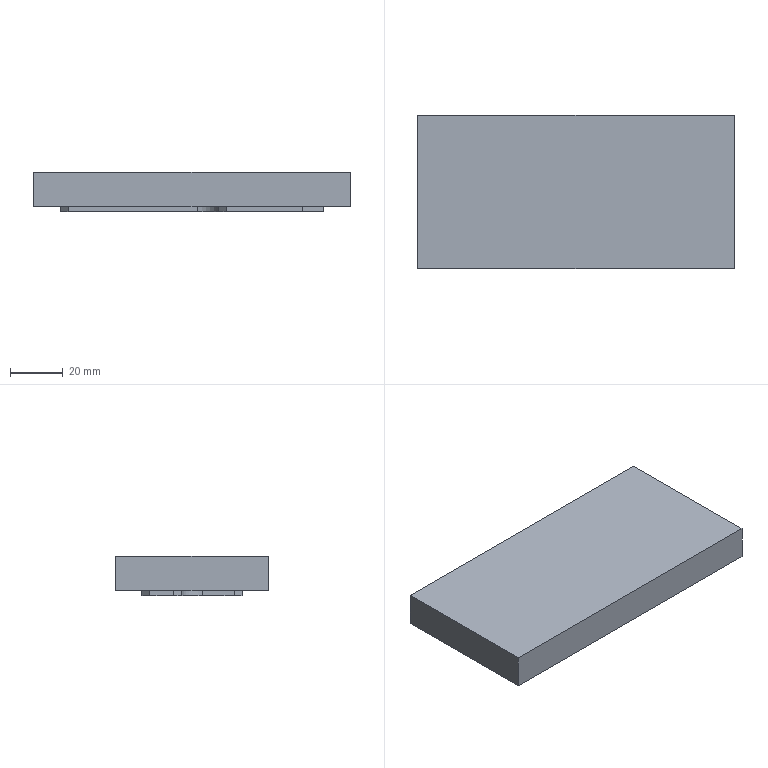NC program | NX | posted with a generic post | part box 120 x 58 x 15 mm
Lines 953 to 1801 of 3687:
(ZLEVEL_PROFILE_COPY_COPY_COPY , TOOL : D3)
N1880 T17 M6
N1882 G54
N1884 G17 G0 G90 X-14.524 Y12.25 S9500 M3
N1886 G43 Z30. H17
N1888 Z1.
N1890 G94 G1 X6.072 Z-0.079 F1000.
N1892 X6.264 Y12.287 Z-0.09
N1894 X6.517 Y12.443 Z-0.105
N1896 X6.691 Y12.683 Z-0.121
N1898 X6.759 Y12.971 Z-0.136
N1900 X6.713 Y13.264 Z-0.152
N1902 X6.591 Y13.477 Z-0.165
N1904 X6.382 Y13.657 Z-0.179
N1906 X6.123 Y13.75 Z-0.194
N1908 X6. Z-0.2
N1910 X-44. F1200.
N1912 G3 X-44.75 Y13. R0.75
N1914 X-44. Y12.25 R0.75
N1916 G1 X6.
N1918 G3 X6.75 Y13. R0.75
N1920 X6. Y13.75 R0.75
N1922 G1 X-5.458 Z-0.4
N1924 X-44.
N1926 G3 X-44.75 Y13. R0.75
N1928 X-44. Y12.25 R0.75
N1930 G1 X6.
N1932 G3 X6.75 Y13. R0.75
N1934 X6. Y13.75 R0.75
N1936 G1 X-5.458 Z-0.6
N1938 X-44.
N1940 G3 X-44.75 Y13. R0.75
N1942 X-44. Y12.25 R0.75
N1944 G1 X6.
N1946 G3 X6.75 Y13. R0.75
N1948 X6. Y13.75 R0.75
N1950 G1 X-5.458 Z-0.8
N1952 X-44.
N1954 G3 X-44.75 Y13. R0.75
N1956 X-44. Y12.25 R0.75
N1958 G1 X6.
N1960 G3 X6.75 Y13. R0.75
N1962 X6. Y13.75 R0.75
N1964 G1 X-5.458 Z-1.
N1966 X-44.
N1968 G3 X-44.75 Y13. R0.75
N1970 X-44. Y12.25 R0.75
N1972 G1 X6.
N1974 G3 X6.75 Y13. R0.75
N1976 X6. Y13.75 R0.75
N1978 G1 X-5.458 Z-1.2
N1980 X-44.
N1982 G3 X-44.75 Y13. R0.75
N1984 X-44. Y12.25 R0.75
N1986 G1 X6.
N1988 G3 X6.75 Y13. R0.75
N1990 X6. Y13.75 R0.75
N1992 G1 X-5.458 Z-1.4
N1994 X-44.
N1996 G3 X-44.75 Y13. R0.75
N1998 X-44. Y12.25 R0.75
N2000 G1 X6.
N2002 G3 X6.75 Y13. R0.75
N2004 X6. Y13.75 R0.75
N2006 G1 X-5.458 Z-1.6
N2008 X-44.
N2010 G3 X-44.75 Y13. R0.75
N2012 X-44. Y12.25 R0.75
N2014 G1 X6.
N2016 G3 X6.75 Y13. R0.75
N2018 X6. Y13.75 R0.75
N2020 G1 X-5.458 Z-1.8
N2022 X-44.
N2024 G3 X-44.75 Y13. R0.75
N2026 X-44. Y12.25 R0.75
N2028 G1 X6.
N2030 G3 X6.75 Y13. R0.75
N2032 X6. Y13.75 R0.75
N2034 G1 X-5.458 Z-2.
N2036 X-44.
N2038 G3 X-44.75 Y13. R0.75
N2040 X-44. Y12.25 R0.75
N2042 G1 X6.
N2044 G3 X6.75 Y13. R0.75
N2046 X6. Y13.75 R0.75
N2048 G1 X-5.458 Z-2.2
N2050 X-44.
N2052 G3 X-44.75 Y13. R0.75
N2054 X-44. Y12.25 R0.75
N2056 G1 X6.
N2058 G3 X6.75 Y13. R0.75
N2060 X6. Y13.75 R0.75
N2062 G1 X-5.458 Z-2.4
N2064 X-44.
N2066 G3 X-44.75 Y13. R0.75
N2068 X-44. Y12.25 R0.75
N2070 G1 X6.
N2072 G3 X6.75 Y13. R0.75
N2074 X6. Y13.75 R0.75
N2076 G1 X-5.458 Z-2.6
N2078 X-44.
N2080 G3 X-44.75 Y13. R0.75
N2082 X-44. Y12.25 R0.75
N2084 G1 X6.
N2086 G3 X6.75 Y13. R0.75
N2088 X6. Y13.75 R0.75
N2090 G1 X-5.458 Z-2.8
N2092 X-44.
N2094 G3 X-44.75 Y13. R0.75
N2096 X-44. Y12.25 R0.75
N2098 G1 X6.
N2100 G3 X6.75 Y13. R0.75
N2102 X6. Y13.75 R0.75
N2104 G1 X-5.458 Z-3.
N2106 X-44.
N2108 G3 X-44.75 Y13. R0.75
N2110 X-44. Y12.25 R0.75
N2112 G1 X6.
N2114 G3 X6.75 Y13. R0.75
N2116 X6. Y13.75 R0.75
N2118 G1 X-5.458 Z-3.2
N2120 X-44.
N2122 G3 X-44.75 Y13. R0.75
N2124 X-44. Y12.25 R0.75
N2126 G1 X6.
N2128 G3 X6.75 Y13. R0.75
N2130 X6. Y13.75 R0.75
N2132 G1 X-5.458 Z-3.4
N2134 X-44.
N2136 G3 X-44.75 Y13. R0.75
N2138 X-44. Y12.25 R0.75
N2140 G1 X6.
N2142 G3 X6.75 Y13. R0.75
N2144 X6. Y13.75 R0.75
N2146 G1 X-5.458 Z-3.6
N2148 X-44.
N2150 G3 X-44.75 Y13. R0.75
N2152 X-44. Y12.25 R0.75
N2154 G1 X6.
N2156 G3 X6.75 Y13. R0.75
N2158 X6. Y13.75 R0.75
N2160 G1 X-5.458 Z-3.8
N2162 X-44.
N2164 G3 X-44.75 Y13. R0.75
N2166 X-44. Y12.25 R0.75
N2168 G1 X6.
N2170 G3 X6.75 Y13. R0.75
N2172 X6. Y13.75 R0.75
N2174 G1 X-5.458 Z-4.
N2176 X-44.
N2178 G3 X-44.75 Y13. R0.75
N2180 X-44. Y12.25 R0.75
N2182 G1 X6.
N2184 G3 X6.75 Y13. R0.75
N2186 X6. Y13.75 R0.75
N2188 G1 X-5.458 Z-4.2
N2190 X-44.
N2192 G3 X-44.75 Y13. R0.75
N2194 X-44. Y12.25 R0.75
N2196 G1 X6.
N2198 G3 X6.75 Y13. R0.75
N2200 X6. Y13.75 R0.75
N2202 G1 X-5.458 Z-4.4
N2204 X-44.
N2206 G3 X-44.75 Y13. R0.75
N2208 X-44. Y12.25 R0.75
N2210 G1 X6.
N2212 G3 X6.75 Y13. R0.75
N2214 X6. Y13.75 R0.75
N2216 G1 X-5.458 Z-4.6
N2218 X-44.
N2220 G3 X-44.75 Y13. R0.75
N2222 X-44. Y12.25 R0.75
N2224 G1 X6.
N2226 G3 X6.75 Y13. R0.75
N2228 X6. Y13.75 R0.75
N2230 G1 X-5.458 Z-4.8
N2232 X-44.
N2234 G3 X-44.75 Y13. R0.75
N2236 X-44. Y12.25 R0.75
N2238 G1 X6.
N2240 G3 X6.75 Y13. R0.75
N2242 X6. Y13.75 R0.75
N2244 G1 X-5.458 Z-5.
N2246 X-44.
N2248 G3 X-44.75 Y13. R0.75
N2250 X-44. Y12.25 R0.75
N2252 G1 X6.
N2254 G3 X6.75 Y13. R0.75
N2256 X6. Y13.75 R0.75
N2258 G1 X-5.458
N2260 G3 X-5.718 Y13.6 R0.3
N2262 G1 X-5.804 Y13.45
N2264 Z-3.2
N2266 G0 Z30.
N2268 X43.738 Y0.489
N2270 Z1.
N2272 G1 X43.759 Y0.135 Z0.981 F1000.
N2274 X43.7 Y-1.278 Z0.907
N2276 X43.497 Y-2.678 Z0.833
N2278 X43.151 Y-4.049 Z0.759
N2280 X42.666 Y-5.378 Z0.685
N2282 X42.047 Y-6.65 Z0.611
N2284 X41.3 Y-7.851 Z0.537
N2286 X40.435 Y-8.97 Z0.463
N2288 X39.459 Y-9.993 Z0.388
N2290 X38.383 Y-10.911 Z0.314
N2292 X37.219 Y-11.714 Z0.24
N2294 X35.978 Y-12.393 Z0.166
N2296 X34.675 Y-12.942 Z0.092
N2298 X33.321 Y-13.353 Z0.018
N2300 X31.933 Y-13.624 Z-0.056
N2302 X30.525 Y-13.75 Z-0.13
N2304 X29.929 Z-0.162
N2306 X29.805 Y-13.828 Z-0.169
N2308 X29.744 Y-13.957 Z-0.177
N2310 X29.78 Y-14.139 Z-0.187
N2312 X29.929 Y-14.25 Z-0.196
N2314 X30. Z-0.2
N2316 G3 X44.25 Y0. R14.25 F1200.
N2318 X30. Y14.25 R14.25
N2320 X29.75 Y14. R0.25
N2322 X30. Y13.75 R0.25
N2324 G2 X43.75 Y0. R13.75
N2326 X30. Y-13.75 R13.75
N2328 G3 X29.75 Y-14. R0.25
N2330 X30. Y-14.25 R0.25
N2332 G1 X30.122 Y-14.246 Z-0.202
N2334 X30.244 Y-14.242 Z-0.204
N2336 X30.365 Y-14.238 Z-0.206
N2338 X30.487 Y-14.232 Z-0.209
N2340 X30.609 Y-14.229 Z-0.211
N2342 X30.731 Y-14.224 Z-0.213
N2344 X30.853 Y-14.221 Z-0.215
N2346 X30.974 Y-14.217 Z-0.217
N2348 X31.096 Y-14.205 Z-0.219
N2350 X31.217 Y-14.192 Z-0.221
N2352 X31.338 Y-14.179 Z-0.223
N2354 X31.459 Y-14.167 Z-0.226
N2356 X31.58 Y-14.154 Z-0.228
N2358 X31.702 Y-14.14 Z-0.23
N2360 X31.823 Y-14.128 Z-0.232
N2362 X31.944 Y-14.115 Z-0.234
N2364 X32.065 Y-14.097 Z-0.236
N2366 X32.185 Y-14.076 Z-0.238
N2368 X32.305 Y-14.055 Z-0.24
N2370 X32.425 Y-14.034 Z-0.243
N2372 X32.545 Y-14.012 Z-0.245
N2374 X32.664 Y-13.991 Z-0.247
N2376 X32.785 Y-13.971 Z-0.249
N2378 X32.905 Y-13.949 Z-0.251
N2380 X33.024 Y-13.924 Z-0.253
N2382 X33.142 Y-13.893 Z-0.255
N2384 X33.26 Y-13.865 Z-0.257
N2386 X33.379 Y-13.836 Z-0.26
N2388 X33.497 Y-13.806 Z-0.262
N2390 X33.615 Y-13.776 Z-0.264
N2392 X33.733 Y-13.747 Z-0.266
N2394 X33.852 Y-13.718 Z-0.268
N2396 X33.969 Y-13.685 Z-0.27
N2398 X34.085 Y-13.648 Z-0.272
N2400 X34.201 Y-13.61 Z-0.274
N2402 X34.317 Y-13.572 Z-0.277
N2404 X34.433 Y-13.534 Z-0.279
N2406 X34.548 Y-13.497 Z-0.281
N2408 X34.664 Y-13.459 Z-0.283
N2410 X34.78 Y-13.42 Z-0.285
N2412 X34.896 Y-13.382 Z-0.287
N2414 X35.009 Y-13.337 Z-0.289
N2416 X35.122 Y-13.291 Z-0.291
N2418 X35.235 Y-13.245 Z-0.294
N2420 X35.348 Y-13.199 Z-0.296
N2422 X35.461 Y-13.154 Z-0.298
N2424 X35.574 Y-13.109 Z-0.3
N2426 X35.686 Y-13.062 Z-0.302
N2428 X35.799 Y-13.016 Z-0.304
N2430 X35.909 Y-12.963 Z-0.306
N2432 X36.019 Y-12.91 Z-0.309
N2434 X36.128 Y-12.856 Z-0.311
N2436 X36.238 Y-12.803 Z-0.313
N2438 X36.347 Y-12.75 Z-0.315
N2440 X36.457 Y-12.696 Z-0.317
N2442 X36.566 Y-12.643 Z-0.319
N2444 X36.676 Y-12.589 Z-0.321
N2446 X36.782 Y-12.529 Z-0.323
N2448 X36.888 Y-12.469 Z-0.326
N2450 X36.993 Y-12.407 Z-0.328
N2452 X37.098 Y-12.346 Z-0.33
N2454 X37.204 Y-12.286 Z-0.332
N2456 X37.31 Y-12.225 Z-0.334
N2458 X37.415 Y-12.164 Z-0.336
N2460 X37.521 Y-12.103 Z-0.338
N2462 X37.623 Y-12.037 Z-0.34
N2464 X37.724 Y-11.968 Z-0.343
N2466 X37.825 Y-11.9 Z-0.345
N2468 X37.926 Y-11.832 Z-0.347
N2470 X38.027 Y-11.764 Z-0.349
N2472 X38.128 Y-11.696 Z-0.351
N2474 X38.229 Y-11.627 Z-0.353
N2476 X38.33 Y-11.56 Z-0.355
N2478 X38.429 Y-11.488 Z-0.357
N2480 X38.525 Y-11.413 Z-0.36
N2482 X38.62 Y-11.337 Z-0.362
N2484 X38.717 Y-11.263 Z-0.364
N2486 X38.813 Y-11.188 Z-0.366
N2488 X38.909 Y-11.112 Z-0.368
N2490 X39.004 Y-11.037 Z-0.37
N2492 X39.101 Y-10.962 Z-0.372
N2494 X39.194 Y-10.885 Z-0.374
N2496 X39.285 Y-10.804 Z-0.377
N2498 X39.375 Y-10.721 Z-0.379
N2500 X39.466 Y-10.64 Z-0.381
N2502 X39.557 Y-10.559 Z-0.383
N2504 X39.648 Y-10.477 Z-0.385
N2506 X39.738 Y-10.396 Z-0.387
N2508 X39.829 Y-10.314 Z-0.389
N2510 X39.918 Y-10.232 Z-0.391
N2512 X40.003 Y-10.144 Z-0.394
N2514 X40.087 Y-10.055 Z-0.396
N2516 X40.172 Y-9.968 Z-0.398
N2518 X40.263 Y-9.886 Z-0.4
N2520 G3 X30. Y14.25 R14.25
N2522 X29.75 Y14. R0.25
N2524 X30. Y13.75 R0.25
N2526 G2 X43.75 Y0. R13.75
N2528 X30. Y-13.75 R13.75
N2530 G3 X29.75 Y-14. R0.25
N2532 X30. Y-14.25 R0.25
N2534 G1 X30.122 Y-14.246 Z-0.402
N2536 X30.244 Y-14.242 Z-0.404
N2538 X30.365 Y-14.238 Z-0.406
N2540 X30.487 Y-14.232 Z-0.409
N2542 X30.609 Y-14.229 Z-0.411
N2544 X30.731 Y-14.224 Z-0.413
N2546 X30.853 Y-14.221 Z-0.415
N2548 X30.974 Y-14.217 Z-0.417
N2550 X31.096 Y-14.205 Z-0.419
N2552 X31.217 Y-14.192 Z-0.421
N2554 X31.338 Y-14.179 Z-0.423
N2556 X31.459 Y-14.167 Z-0.426
N2558 X31.581 Y-14.154 Z-0.428
N2560 X31.702 Y-14.14 Z-0.43
N2562 X31.823 Y-14.128 Z-0.432
N2564 X31.944 Y-14.115 Z-0.434
N2566 X32.065 Y-14.097 Z-0.436
N2568 X32.185 Y-14.076 Z-0.438
N2570 X32.305 Y-14.055 Z-0.44
N2572 X32.425 Y-14.034 Z-0.443
N2574 X32.545 Y-14.012 Z-0.445
N2576 X32.664 Y-13.991 Z-0.447
N2578 X32.785 Y-13.971 Z-0.449
N2580 X32.905 Y-13.949 Z-0.451
N2582 X33.024 Y-13.924 Z-0.453
N2584 X33.142 Y-13.893 Z-0.455
N2586 X33.26 Y-13.865 Z-0.457
N2588 X33.379 Y-13.836 Z-0.46
N2590 X33.497 Y-13.806 Z-0.462
N2592 X33.615 Y-13.776 Z-0.464
N2594 X33.733 Y-13.747 Z-0.466
N2596 X33.852 Y-13.718 Z-0.468
N2598 X33.969 Y-13.685 Z-0.47
N2600 X34.085 Y-13.648 Z-0.472
N2602 X34.201 Y-13.61 Z-0.474
N2604 X34.317 Y-13.572 Z-0.477
N2606 X34.433 Y-13.534 Z-0.479
N2608 X34.548 Y-13.497 Z-0.481
N2610 X34.664 Y-13.459 Z-0.483
N2612 X34.78 Y-13.42 Z-0.485
N2614 X34.896 Y-13.382 Z-0.487
N2616 X35.009 Y-13.337 Z-0.489
N2618 X35.122 Y-13.291 Z-0.491
N2620 X35.235 Y-13.245 Z-0.494
N2622 X35.348 Y-13.199 Z-0.496
N2624 X35.461 Y-13.154 Z-0.498
N2626 X35.574 Y-13.109 Z-0.5
N2628 X35.686 Y-13.062 Z-0.502
N2630 X35.799 Y-13.016 Z-0.504
N2632 X35.909 Y-12.963 Z-0.506
N2634 X36.019 Y-12.91 Z-0.509
N2636 X36.128 Y-12.856 Z-0.511
N2638 X36.238 Y-12.803 Z-0.513
N2640 X36.347 Y-12.75 Z-0.515
N2642 X36.457 Y-12.696 Z-0.517
N2644 X36.566 Y-12.643 Z-0.519
N2646 X36.676 Y-12.589 Z-0.521
N2648 X36.782 Y-12.529 Z-0.523
N2650 X36.888 Y-12.469 Z-0.526
N2652 X36.993 Y-12.407 Z-0.528
N2654 X37.098 Y-12.346 Z-0.53
N2656 X37.204 Y-12.286 Z-0.532
N2658 X37.31 Y-12.225 Z-0.534
N2660 X37.415 Y-12.164 Z-0.536
N2662 X37.521 Y-12.103 Z-0.538
N2664 X37.623 Y-12.037 Z-0.54
N2666 X37.724 Y-11.968 Z-0.543
N2668 X37.825 Y-11.9 Z-0.545
N2670 X37.926 Y-11.832 Z-0.547
N2672 X38.027 Y-11.764 Z-0.549
N2674 X38.128 Y-11.696 Z-0.551
N2676 X38.229 Y-11.627 Z-0.553
N2678 X38.33 Y-11.56 Z-0.555
N2680 X38.429 Y-11.488 Z-0.557
N2682 X38.525 Y-11.413 Z-0.56
N2684 X38.62 Y-11.337 Z-0.562
N2686 X38.717 Y-11.262 Z-0.564
N2688 X38.813 Y-11.188 Z-0.566
N2690 X38.909 Y-11.112 Z-0.568
N2692 X39.004 Y-11.037 Z-0.57
N2694 X39.101 Y-10.962 Z-0.572
N2696 X39.194 Y-10.885 Z-0.574
N2698 X39.285 Y-10.804 Z-0.577
N2700 X39.375 Y-10.721 Z-0.579
N2702 X39.466 Y-10.64 Z-0.581
N2704 X39.557 Y-10.559 Z-0.583
N2706 X39.648 Y-10.477 Z-0.585
N2708 X39.738 Y-10.396 Z-0.587
N2710 X39.829 Y-10.314 Z-0.589
N2712 X39.918 Y-10.232 Z-0.591
N2714 X40.003 Y-10.144 Z-0.594
N2716 X40.087 Y-10.055 Z-0.596
N2718 X40.172 Y-9.968 Z-0.598
N2720 X40.263 Y-9.886 Z-0.6
N2722 G3 X30. Y14.25 R14.25
N2724 X29.75 Y14. R0.25
N2726 X30. Y13.75 R0.25
N2728 G2 X43.75 Y0. R13.75
N2730 X30. Y-13.75 R13.75
N2732 G3 X29.75 Y-14. R0.25
N2734 X30. Y-14.25 R0.25
N2736 G1 X30.122 Y-14.246 Z-0.602
N2738 X30.244 Y-14.242 Z-0.604
N2740 X30.365 Y-14.238 Z-0.606
N2742 X30.487 Y-14.232 Z-0.609
N2744 X30.609 Y-14.229 Z-0.611
N2746 X30.731 Y-14.224 Z-0.613
N2748 X30.853 Y-14.221 Z-0.615
N2750 X30.974 Y-14.217 Z-0.617
N2752 X31.096 Y-14.205 Z-0.619
N2754 X31.217 Y-14.192 Z-0.621
N2756 X31.338 Y-14.179 Z-0.623
N2758 X31.459 Y-14.167 Z-0.626
N2760 X31.581 Y-14.154 Z-0.628
N2762 X31.702 Y-14.14 Z-0.63
N2764 X31.823 Y-14.128 Z-0.632
N2766 X31.944 Y-14.115 Z-0.634
N2768 X32.065 Y-14.097 Z-0.636
N2770 X32.185 Y-14.076 Z-0.638
N2772 X32.305 Y-14.055 Z-0.64
N2774 X32.425 Y-14.034 Z-0.643
N2776 X32.545 Y-14.012 Z-0.645
N2778 X32.664 Y-13.991 Z-0.647
N2780 X32.785 Y-13.971 Z-0.649
N2782 X32.905 Y-13.949 Z-0.651
N2784 X33.024 Y-13.924 Z-0.653
N2786 X33.142 Y-13.893 Z-0.655
N2788 X33.26 Y-13.865 Z-0.657
N2790 X33.379 Y-13.836 Z-0.66
N2792 X33.497 Y-13.806 Z-0.662
N2794 X33.615 Y-13.776 Z-0.664
N2796 X33.733 Y-13.747 Z-0.666
N2798 X33.852 Y-13.718 Z-0.668
N2800 X33.969 Y-13.685 Z-0.67
N2802 X34.085 Y-13.648 Z-0.672
N2804 X34.201 Y-13.61 Z-0.674
N2806 X34.317 Y-13.572 Z-0.677
N2808 X34.433 Y-13.534 Z-0.679
N2810 X34.548 Y-13.497 Z-0.681
N2812 X34.664 Y-13.459 Z-0.683
N2814 X34.78 Y-13.42 Z-0.685
N2816 X34.896 Y-13.382 Z-0.687
N2818 X35.009 Y-13.337 Z-0.689
N2820 X35.122 Y-13.291 Z-0.691
N2822 X35.235 Y-13.245 Z-0.694
N2824 X35.348 Y-13.199 Z-0.696
N2826 X35.461 Y-13.154 Z-0.698
N2828 X35.574 Y-13.109 Z-0.7
N2830 X35.686 Y-13.062 Z-0.702
N2832 X35.799 Y-13.016 Z-0.704
N2834 X35.909 Y-12.963 Z-0.706
N2836 X36.019 Y-12.91 Z-0.709
N2838 X36.128 Y-12.856 Z-0.711
N2840 X36.238 Y-12.803 Z-0.713
N2842 X36.347 Y-12.75 Z-0.715
N2844 X36.457 Y-12.696 Z-0.717
N2846 X36.566 Y-12.643 Z-0.719
N2848 X36.676 Y-12.589 Z-0.721
N2850 X36.782 Y-12.529 Z-0.723
N2852 X36.888 Y-12.469 Z-0.726
N2854 X36.993 Y-12.407 Z-0.728
N2856 X37.098 Y-12.346 Z-0.73
N2858 X37.204 Y-12.286 Z-0.732
N2860 X37.31 Y-12.225 Z-0.734
N2862 X37.415 Y-12.164 Z-0.736
N2864 X37.521 Y-12.103 Z-0.738
N2866 X37.623 Y-12.037 Z-0.74
N2868 X37.724 Y-11.968 Z-0.743
N2870 X37.825 Y-11.9 Z-0.745
N2872 X37.926 Y-11.832 Z-0.747
N2874 X38.027 Y-11.764 Z-0.749
N2876 X38.128 Y-11.696 Z-0.751
N2878 X38.229 Y-11.627 Z-0.753
N2880 X38.33 Y-11.56 Z-0.755
N2882 X38.429 Y-11.488 Z-0.757
N2884 X38.525 Y-11.413 Z-0.76
N2886 X38.62 Y-11.337 Z-0.762
N2888 X38.717 Y-11.262 Z-0.764
N2890 X38.813 Y-11.188 Z-0.766
N2892 X38.909 Y-11.112 Z-0.768
N2894 X39.004 Y-11.037 Z-0.77
N2896 X39.101 Y-10.962 Z-0.772
N2898 X39.194 Y-10.885 Z-0.774
N2900 X39.285 Y-10.803 Z-0.777
N2902 X39.375 Y-10.721 Z-0.779
N2904 X39.466 Y-10.64 Z-0.781
N2906 X39.557 Y-10.559 Z-0.783
N2908 X39.648 Y-10.477 Z-0.785
N2910 X39.738 Y-10.396 Z-0.787
N2912 X39.829 Y-10.314 Z-0.789
N2914 X39.918 Y-10.232 Z-0.791
N2916 X40.003 Y-10.144 Z-0.794
N2918 X40.087 Y-10.055 Z-0.796
N2920 X40.172 Y-9.968 Z-0.798
N2922 X40.263 Y-9.886 Z-0.8
N2924 G3 X30. Y14.25 R14.25
N2926 X29.75 Y14. R0.25
N2928 X30. Y13.75 R0.25
N2930 G2 X43.75 Y0. R13.75
N2932 X30. Y-13.75 R13.75
N2934 G3 X29.75 Y-14. R0.25
N2936 X30. Y-14.25 R0.25
N2938 G1 X30.122 Y-14.246 Z-0.802
N2940 X30.244 Y-14.242 Z-0.804
N2942 X30.365 Y-14.238 Z-0.806
N2944 X30.487 Y-14.232 Z-0.809
N2946 X30.609 Y-14.229 Z-0.811
N2948 X30.731 Y-14.224 Z-0.813
N2950 X30.853 Y-14.221 Z-0.815
N2952 X30.974 Y-14.217 Z-0.817
N2954 X31.096 Y-14.205 Z-0.819
N2956 X31.217 Y-14.192 Z-0.821
N2958 X31.338 Y-14.179 Z-0.823
N2960 X31.459 Y-14.167 Z-0.826
N2962 X31.581 Y-14.154 Z-0.828
N2964 X31.702 Y-14.14 Z-0.83
N2966 X31.823 Y-14.128 Z-0.832
N2968 X31.944 Y-14.115 Z-0.834
N2970 X32.065 Y-14.097 Z-0.836
N2972 X32.185 Y-14.076 Z-0.838
N2974 X32.305 Y-14.055 Z-0.84
N2976 X32.425 Y-14.034 Z-0.843
N2978 X32.545 Y-14.012 Z-0.845
N2980 X32.664 Y-13.991 Z-0.847
N2982 X32.785 Y-13.971 Z-0.849
N2984 X32.905 Y-13.949 Z-0.851
N2986 X33.024 Y-13.924 Z-0.853
N2988 X33.142 Y-13.893 Z-0.855
N2990 X33.26 Y-13.865 Z-0.857
N2992 X33.379 Y-13.836 Z-0.86
N2994 X33.497 Y-13.806 Z-0.862
N2996 X33.615 Y-13.776 Z-0.864
N2998 X33.733 Y-13.747 Z-0.866
N3000 X33.852 Y-13.718 Z-0.868
N3002 X33.969 Y-13.685 Z-0.87
N3004 X34.085 Y-13.648 Z-0.872
N3006 X34.201 Y-13.61 Z-0.874
N3008 X34.317 Y-13.572 Z-0.877
N3010 X34.433 Y-13.534 Z-0.879
N3012 X34.548 Y-13.497 Z-0.881
N3014 X34.664 Y-13.459 Z-0.883
N3016 X34.78 Y-13.42 Z-0.885
N3018 X34.896 Y-13.382 Z-0.887
N3020 X35.009 Y-13.337 Z-0.889
N3022 X35.122 Y-13.291 Z-0.891
N3024 X35.235 Y-13.245 Z-0.894
N3026 X35.348 Y-13.199 Z-0.896
N3028 X35.461 Y-13.154 Z-0.898
N3030 X35.574 Y-13.109 Z-0.9
N3032 X35.686 Y-13.062 Z-0.902
N3034 X35.799 Y-13.016 Z-0.904
N3036 X35.909 Y-12.963 Z-0.906
N3038 X36.019 Y-12.91 Z-0.909
N3040 X36.128 Y-12.856 Z-0.911
N3042 X36.238 Y-12.803 Z-0.913
N3044 X36.347 Y-12.75 Z-0.915
N3046 X36.457 Y-12.696 Z-0.917
N3048 X36.566 Y-12.643 Z-0.919
N3050 X36.676 Y-12.589 Z-0.921
N3052 X36.782 Y-12.529 Z-0.923
N3054 X36.888 Y-12.469 Z-0.926
N3056 X36.993 Y-12.407 Z-0.928
N3058 X37.098 Y-12.346 Z-0.93
N3060 X37.204 Y-12.286 Z-0.932
N3062 X37.31 Y-12.225 Z-0.934
N3064 X37.415 Y-12.164 Z-0.936
N3066 X37.521 Y-12.103 Z-0.938
N3068 X37.623 Y-12.037 Z-0.94
N3070 X37.724 Y-11.968 Z-0.943
N3072 X37.825 Y-11.9 Z-0.945
N3074 X37.926 Y-11.832 Z-0.947
N3076 X38.027 Y-11.764 Z-0.949
N3078 X38.128 Y-11.696 Z-0.951
N3080 X38.229 Y-11.627 Z-0.953
N3082 X38.33 Y-11.56 Z-0.955
N3084 X38.429 Y-11.488 Z-0.957
N3086 X38.525 Y-11.413 Z-0.96
N3088 X38.62 Y-11.337 Z-0.962
N3090 X38.717 Y-11.262 Z-0.964
N3092 X38.813 Y-11.188 Z-0.966
N3094 X38.909 Y-11.112 Z-0.968
N3096 X39.004 Y-11.037 Z-0.97
N3098 X39.101 Y-10.962 Z-0.972
N3100 X39.194 Y-10.885 Z-0.974
N3102 X39.285 Y-10.803 Z-0.977
N3104 X39.375 Y-10.721 Z-0.979
N3106 X39.467 Y-10.641 Z-0.981
N3108 X39.557 Y-10.559 Z-0.983
N3110 X39.648 Y-10.477 Z-0.985
N3112 X39.738 Y-10.396 Z-0.987
N3114 X39.829 Y-10.314 Z-0.989
N3116 X39.918 Y-10.232 Z-0.991
N3118 X40.003 Y-10.144 Z-0.994
N3120 X40.087 Y-10.055 Z-0.996
N3122 X40.172 Y-9.968 Z-0.998
N3124 X40.263 Y-9.886 Z-1.
N3126 G3 X30. Y14.25 R14.25
N3128 X29.75 Y14. R0.25
N3130 X30. Y13.75 R0.25
N3132 G2 X43.75 Y0. R13.75
N3134 X30. Y-13.75 R13.75
N3136 G3 X29.75 Y-14. R0.25
N3138 X30. Y-14.25 R0.25
N3140 G1 X30.122 Y-14.246 Z-1.002
N3142 X30.244 Y-14.242 Z-1.004
N3144 X30.365 Y-14.238 Z-1.006
N3146 X30.487 Y-14.232 Z-1.009
N3148 X30.609 Y-14.229 Z-1.011
N3150 X30.731 Y-14.224 Z-1.013
N3152 X30.853 Y-14.221 Z-1.015
N3154 X30.974 Y-14.217 Z-1.017
N3156 X31.096 Y-14.205 Z-1.019
N3158 X31.217 Y-14.192 Z-1.021
N3160 X31.338 Y-14.179 Z-1.023
N3162 X31.459 Y-14.167 Z-1.026
N3164 X31.581 Y-14.154 Z-1.028
N3166 X31.702 Y-14.14 Z-1.03
N3168 X31.823 Y-14.128 Z-1.032
N3170 X31.944 Y-14.115 Z-1.034
N3172 X32.065 Y-14.097 Z-1.036
N3174 X32.185 Y-14.076 Z-1.038
N3176 X32.305 Y-14.055 Z-1.04
N3178 X32.425 Y-14.034 Z-1.043
N3180 X32.545 Y-14.012 Z-1.045
N3182 X32.664 Y-13.991 Z-1.047
N3184 X32.785 Y-13.971 Z-1.049
N3186 X32.905 Y-13.949 Z-1.051
N3188 X33.024 Y-13.924 Z-1.053
N3190 X33.142 Y-13.893 Z-1.055
N3192 X33.26 Y-13.865 Z-1.057
N3194 X33.379 Y-13.836 Z-1.06
N3196 X33.497 Y-13.806 Z-1.062
N3198 X33.615 Y-13.776 Z-1.064
N3200 X33.733 Y-13.747 Z-1.066
N3202 X33.852 Y-13.717 Z-1.068
N3204 X33.969 Y-13.685 Z-1.07
N3206 X34.085 Y-13.648 Z-1.072
N3208 X34.201 Y-13.61 Z-1.074
N3210 X34.317 Y-13.572 Z-1.077
N3212 X34.433 Y-13.534 Z-1.079
N3214 X34.548 Y-13.497 Z-1.081
N3216 X34.664 Y-13.459 Z-1.083
N3218 X34.78 Y-13.42 Z-1.085
N3220 X34.896 Y-13.382 Z-1.087
N3222 X35.009 Y-13.337 Z-1.089
N3224 X35.122 Y-13.291 Z-1.091
N3226 X35.235 Y-13.245 Z-1.094
N3228 X35.348 Y-13.199 Z-1.096
N3230 X35.461 Y-13.154 Z-1.098
N3232 X35.574 Y-13.109 Z-1.1
N3234 X35.686 Y-13.062 Z-1.102
N3236 X35.799 Y-13.016 Z-1.104
N3238 X35.909 Y-12.963 Z-1.106
N3240 X36.019 Y-12.91 Z-1.109
N3242 X36.128 Y-12.856 Z-1.111
N3244 X36.238 Y-12.803 Z-1.113
N3246 X36.347 Y-12.75 Z-1.115
N3248 X36.457 Y-12.696 Z-1.117
N3250 X36.566 Y-12.643 Z-1.119
N3252 X36.676 Y-12.589 Z-1.121
N3254 X36.782 Y-12.529 Z-1.123
N3256 X36.888 Y-12.469 Z-1.126
N3258 X36.993 Y-12.407 Z-1.128
N3260 X37.098 Y-12.346 Z-1.13
N3262 X37.204 Y-12.286 Z-1.132
N3264 X37.31 Y-12.225 Z-1.134
N3266 X37.415 Y-12.164 Z-1.136
N3268 X37.521 Y-12.103 Z-1.138
N3270 X37.623 Y-12.037 Z-1.14
N3272 X37.724 Y-11.968 Z-1.143
N3274 X37.825 Y-11.9 Z-1.145
N3276 X37.926 Y-11.832 Z-1.147
N3278 X38.027 Y-11.764 Z-1.149
N3280 X38.128 Y-11.696 Z-1.151
N3282 X38.229 Y-11.627 Z-1.153
N3284 X38.33 Y-11.56 Z-1.155
N3286 X38.429 Y-11.488 Z-1.157
N3288 X38.525 Y-11.413 Z-1.16
N3290 X38.62 Y-11.337 Z-1.162
N3292 X38.717 Y-11.262 Z-1.164
N3294 X38.813 Y-11.188 Z-1.166
N3296 X38.909 Y-11.112 Z-1.168
N3298 X39.004 Y-11.037 Z-1.17
N3300 X39.101 Y-10.962 Z-1.172
N3302 X39.194 Y-10.885 Z-1.174
N3304 X39.285 Y-10.803 Z-1.177
N3306 X39.375 Y-10.721 Z-1.179
N3308 X39.467 Y-10.641 Z-1.181
N3310 X39.557 Y-10.559 Z-1.183
N3312 X39.647 Y-10.477 Z-1.185
N3314 X39.738 Y-10.396 Z-1.187
N3316 X39.829 Y-10.314 Z-1.189
N3318 X39.918 Y-10.232 Z-1.191
N3320 X40.003 Y-10.144 Z-1.194
N3322 X40.087 Y-10.055 Z-1.196
N3324 X40.172 Y-9.968 Z-1.198
N3326 X40.263 Y-9.886 Z-1.2
N3328 G3 X30. Y14.25 R14.25
N3330 X29.75 Y14. R0.25
N3332 X30. Y13.75 R0.25
N3334 G2 X43.75 Y0. R13.75
N3336 X30. Y-13.75 R13.75
N3338 G3 X29.75 Y-14. R0.25
N3340 X30. Y-14.25 R0.25
N3342 G1 X30.122 Y-14.246 Z-1.202
N3344 X30.244 Y-14.242 Z-1.204
N3346 X30.365 Y-14.238 Z-1.206
N3348 X30.487 Y-14.232 Z-1.209
N3350 X30.609 Y-14.229 Z-1.211
N3352 X30.731 Y-14.224 Z-1.213
N3354 X30.853 Y-14.221 Z-1.215
N3356 X30.974 Y-14.217 Z-1.217
N3358 X31.096 Y-14.205 Z-1.219
N3360 X31.217 Y-14.192 Z-1.221
N3362 X31.338 Y-14.179 Z-1.223
N3364 X31.459 Y-14.167 Z-1.226
N3366 X31.58 Y-14.154 Z-1.228
N3368 X31.702 Y-14.14 Z-1.23
N3370 X31.823 Y-14.128 Z-1.232
N3372 X31.944 Y-14.115 Z-1.234
N3374 X32.065 Y-14.097 Z-1.236
N3376 X32.185 Y-14.076 Z-1.238
N3378 X32.305 Y-14.055 Z-1.24
N3380 X32.425 Y-14.034 Z-1.243
N3382 X32.545 Y-14.012 Z-1.245
N3384 X32.664 Y-13.991 Z-1.247
N3386 X32.785 Y-13.971 Z-1.249
N3388 X32.905 Y-13.949 Z-1.251
N3390 X33.024 Y-13.924 Z-1.253
N3392 X33.142 Y-13.893 Z-1.255
N3394 X33.26 Y-13.865 Z-1.257
N3396 X33.379 Y-13.836 Z-1.26
N3398 X33.497 Y-13.806 Z-1.262
N3400 X33.615 Y-13.776 Z-1.264
N3402 X33.733 Y-13.747 Z-1.266
N3404 X33.852 Y-13.717 Z-1.268
N3406 X33.969 Y-13.685 Z-1.27
N3408 X34.085 Y-13.648 Z-1.272
N3410 X34.201 Y-13.61 Z-1.274
N3412 X34.317 Y-13.572 Z-1.277
N3414 X34.432 Y-13.534 Z-1.279
N3416 X34.548 Y-13.497 Z-1.281
N3418 X34.664 Y-13.459 Z-1.283
N3420 X34.78 Y-13.42 Z-1.285
N3422 X34.896 Y-13.382 Z-1.287
N3424 X35.009 Y-13.337 Z-1.289
N3426 X35.122 Y-13.291 Z-1.291
N3428 X35.235 Y-13.245 Z-1.294
N3430 X35.348 Y-13.199 Z-1.296
N3432 X35.461 Y-13.154 Z-1.298
N3434 X35.574 Y-13.109 Z-1.3
N3436 X35.686 Y-13.062 Z-1.302
N3438 X35.799 Y-13.016 Z-1.304
N3440 X35.909 Y-12.963 Z-1.306
N3442 X36.019 Y-12.91 Z-1.309
N3444 X36.128 Y-12.856 Z-1.311
N3446 X36.238 Y-12.803 Z-1.313
N3448 X36.347 Y-12.75 Z-1.315
N3450 X36.457 Y-12.696 Z-1.317
N3452 X36.566 Y-12.643 Z-1.319
N3454 X36.676 Y-12.589 Z-1.321
N3456 X36.782 Y-12.529 Z-1.323
N3458 X36.888 Y-12.469 Z-1.326
N3460 X36.993 Y-12.407 Z-1.328
N3462 X37.098 Y-12.346 Z-1.33
N3464 X37.204 Y-12.286 Z-1.332
N3466 X37.31 Y-12.225 Z-1.334
N3468 X37.415 Y-12.164 Z-1.336
N3470 X37.521 Y-12.103 Z-1.338
N3472 X37.623 Y-12.037 Z-1.34
N3474 X37.724 Y-11.968 Z-1.343
N3476 X37.825 Y-11.9 Z-1.345
N3478 X37.926 Y-11.832 Z-1.347
N3480 X38.027 Y-11.764 Z-1.349
N3482 X38.128 Y-11.696 Z-1.351
N3484 X38.229 Y-11.627 Z-1.353
N3486 X38.33 Y-11.56 Z-1.355
N3488 X38.429 Y-11.488 Z-1.357
N3490 X38.525 Y-11.413 Z-1.36
N3492 X38.62 Y-11.337 Z-1.362
N3494 X38.717 Y-11.262 Z-1.364
N3496 X38.813 Y-11.188 Z-1.366
N3498 X38.909 Y-11.112 Z-1.368
N3500 X39.004 Y-11.037 Z-1.37
N3502 X39.101 Y-10.962 Z-1.372
N3504 X39.194 Y-10.885 Z-1.374
N3506 X39.285 Y-10.803 Z-1.377
N3508 X39.375 Y-10.721 Z-1.379
N3510 X39.467 Y-10.641 Z-1.381
N3512 X39.557 Y-10.559 Z-1.383
N3514 X39.647 Y-10.477 Z-1.385
N3516 X39.738 Y-10.396 Z-1.387
N3518 X39.829 Y-10.314 Z-1.389
N3520 X39.918 Y-10.232 Z-1.391
N3522 X40.003 Y-10.144 Z-1.394
N3524 X40.087 Y-10.055 Z-1.396
N3526 X40.172 Y-9.968 Z-1.398
N3528 X40.263 Y-9.886 Z-1.4
N3530 G3 X30. Y14.25 R14.25
N3532 X29.75 Y14. R0.25
N3534 X30. Y13.75 R0.25
N3536 G2 X43.75 Y0. R13.75
N3538 X30. Y-13.75 R13.75
N3540 G3 X29.75 Y-14. R0.25
N3542 X30. Y-14.25 R0.25
N3544 G1 X30.122 Y-14.246 Z-1.402
N3546 X30.244 Y-14.242 Z-1.404
N3548 X30.365 Y-14.238 Z-1.406
N3550 X30.487 Y-14.232 Z-1.409
N3552 X30.609 Y-14.229 Z-1.411
N3554 X30.731 Y-14.224 Z-1.413
N3556 X30.853 Y-14.221 Z-1.415
N3558 X30.974 Y-14.217 Z-1.417
N3560 X31.096 Y-14.205 Z-1.419
N3562 X31.217 Y-14.192 Z-1.421
N3564 X31.338 Y-14.179 Z-1.423
N3566 X31.459 Y-14.167 Z-1.426
N3568 X31.58 Y-14.154 Z-1.428
N3570 X31.702 Y-14.14 Z-1.43